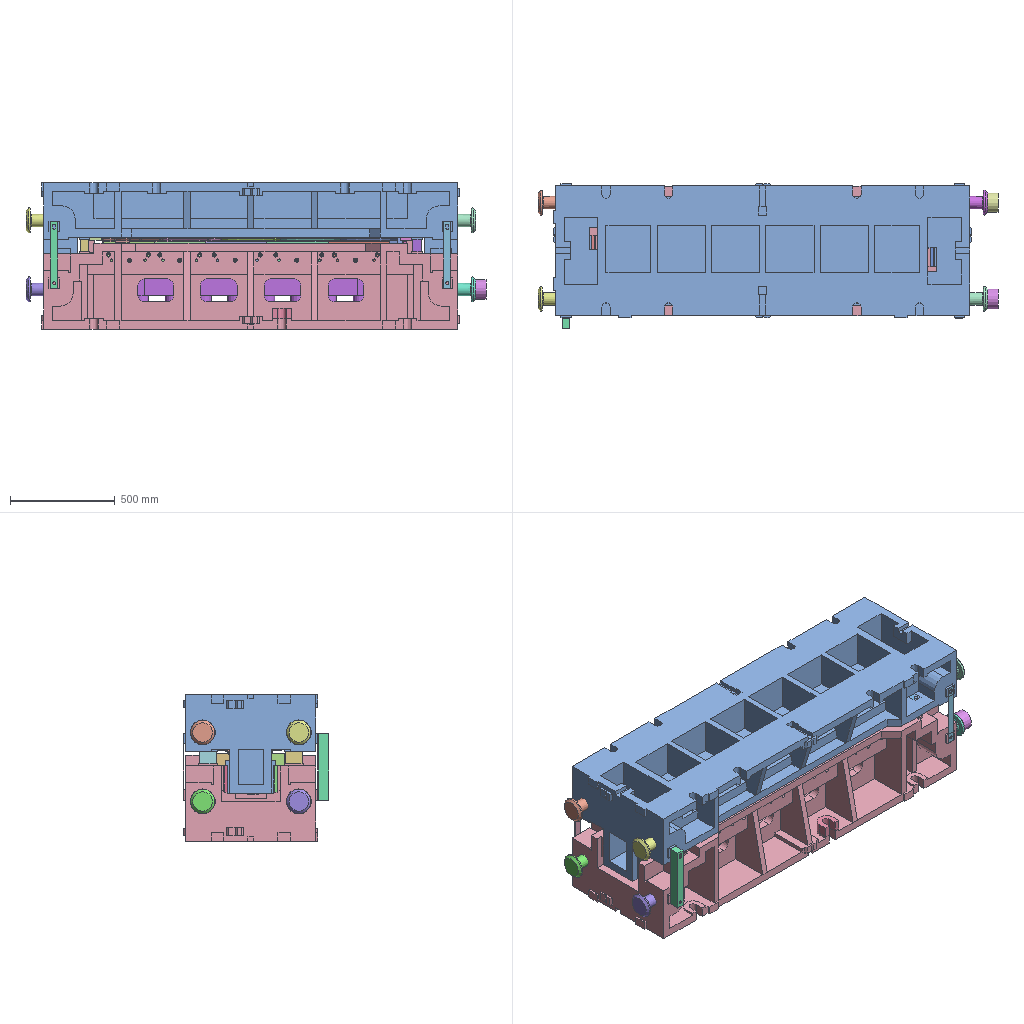Assembly | NX | 102 different items | 102 placed | box 2200 x 696 x 700 mm
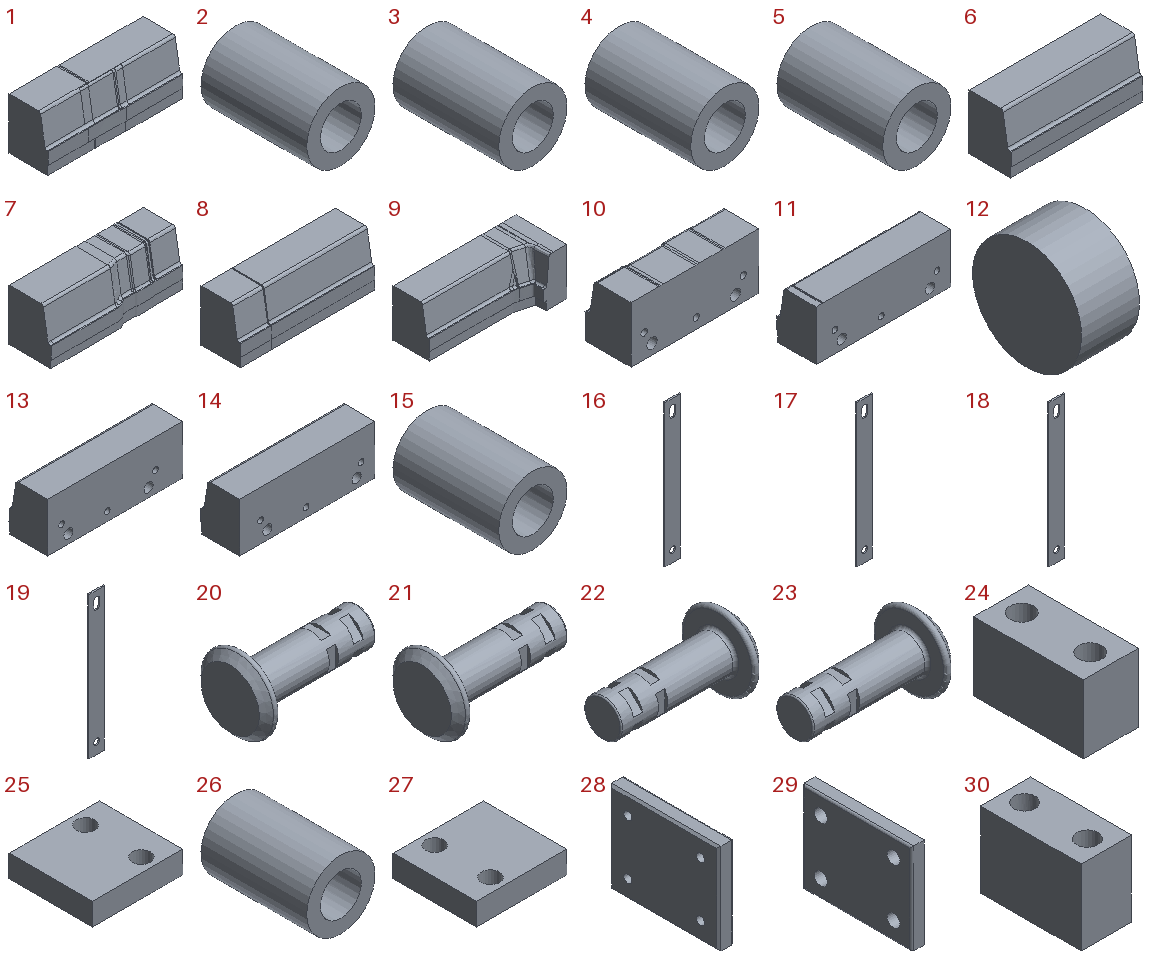Parts list (item | quantity | size | volume | features):
1 | x1 | 280 x 83.171 x 107.133 mm | 2238545 mm3 | features solid 2
2 | x1 | 20 x 31 x 20 mm | 6233 mm3 | features solid 2
3 | x1 | 20 x 31 x 20 mm | 6233 mm3 | features solid 2
4 | x1 | 20 x 31 x 20 mm | 6233 mm3 | features solid 2
5 | x1 | 20 x 31 x 20 mm | 6233 mm3 | features solid 2
6 | x1 | 255 x 82.128 x 107.133 mm | 2023073 mm3 | features solid 2
7 | x1 | 280 x 88.161 x 107.138 mm | 2308062 mm3 | features solid 2
8 | x1 | 280 x 82.346 x 107.138 mm | 2225782 mm3 | features solid 2
9 | x1 | 280 x 116 x 107.135 mm | 2471455 mm3 | features solid 2
10 | x1 | 245 x 88.207 x 107.259 mm | 2041694 mm3 | features solid 2
11 | x1 | 290 x 84.721 x 107.133 mm | 2405435 mm3 | features solid 2
12 | x1 | 50 x 94.142 x 94.142 mm | 348039 mm3 | features solid 2
13 | x1 | 295 x 84.705 x 107.133 mm | 2449051 mm3 | features solid 2
14 | x1 | 295 x 84.706 x 107.133 mm | 2449050 mm3 | features solid 2
15 | x1 | 20 x 31 x 20 mm | 6233 mm3 | features solid 2
16 | x1 | 35 x 3 x 320 mm | 32235 mm3 | features solid 2
17 | x1 | 35 x 3 x 320 mm | 32235 mm3 | features solid 2
18 | x1 | 35 x 3 x 320 mm | 32235 mm3 | features solid 2
19 | x1 | 35 x 3 x 320 mm | 32235 mm3 | features solid 2
20 | x1 | 205 x 120 x 120 mm | 705223 mm3 | features solid 2
21 | x1 | 205 x 120 x 120 mm | 705223 mm3 | features solid 2
22 | x1 | 205 x 120 x 120 mm | 705223 mm3 | features solid 2
23 | x1 | 205 x 120 x 120 mm | 705223 mm3 | features solid 2
24 | x1 | 40 x 80 x 50 mm | 137302 mm3 | features solid 2
25 | x1 | 65 x 60 x 16 mm | 58153 mm3 | features solid 2
26 | x1 | 20 x 31 x 20 mm | 6233 mm3 | features solid 2
27 | x1 | 65 x 60 x 16 mm | 58153 mm3 | features solid 2
28 | x1 | 20 x 150 x 125 mm | 356923 mm3 | features solid 2
29 | x1 | 20 x 150 x 125 mm | 356923 mm3 | features solid 2
30 | x1 | 40 x 80 x 60 mm | 176638 mm3 | features solid 2
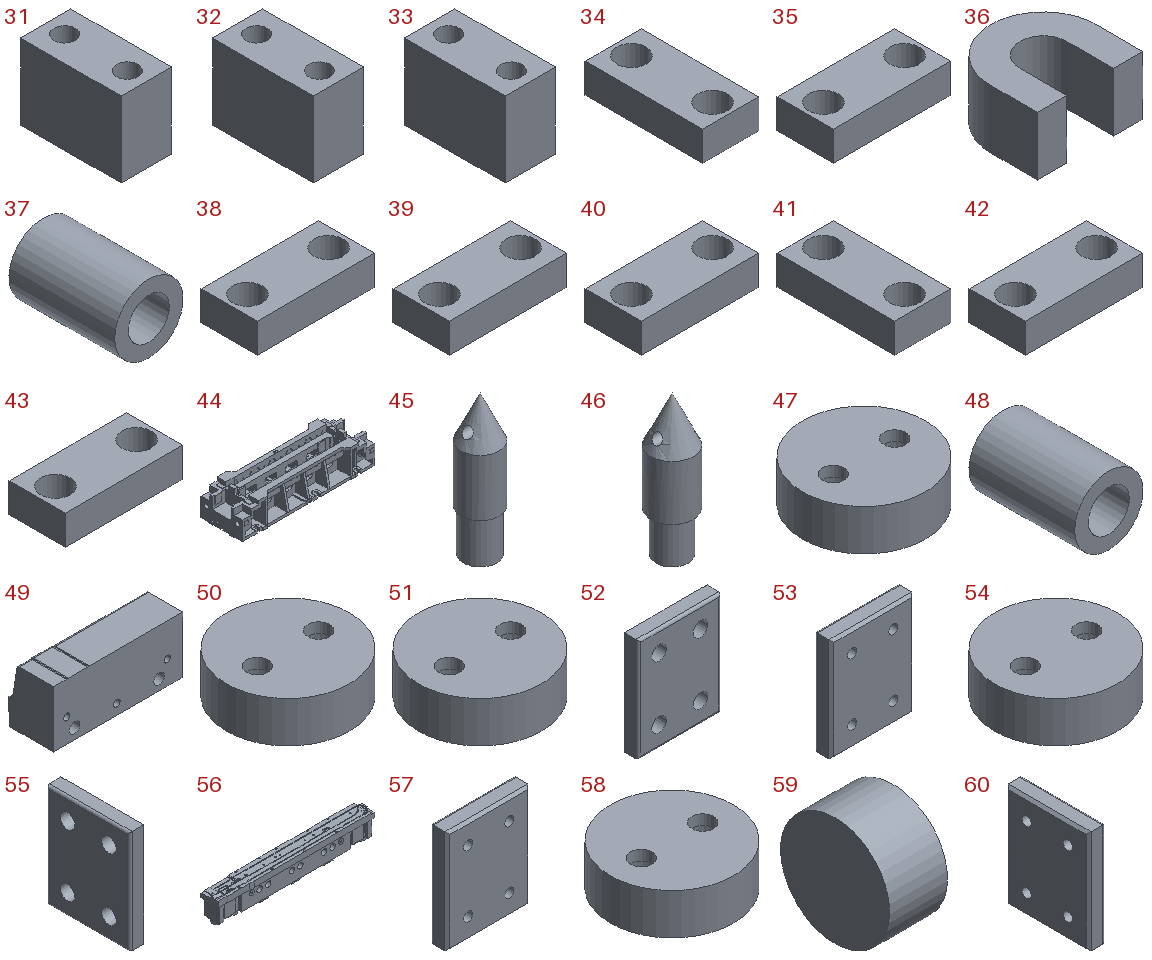31 | x1 | 40 x 80 x 60 mm | 176638 mm3 | features solid 2
32 | x1 | 40 x 80 x 60 mm | 176638 mm3 | features solid 2
33 | x1 | 40 x 80 x 60 mm | 176638 mm3 | features solid 2
34 | x1 | 38 x 80 x 20 mm | 50411 mm3 | features solid 2
35 | x1 | 80 x 38 x 20 mm | 50411 mm3 | features solid 2
36 | x1 | 90 x 85 x 50 mm | 227627 mm3 | features solid 2
37 | x1 | 20 x 31 x 20 mm | 6233 mm3 | features solid 2
38 | x1 | 80 x 38 x 20 mm | 50411 mm3 | features solid 2
39 | x1 | 80 x 38 x 20 mm | 50411 mm3 | features solid 2
40 | x1 | 80 x 38 x 20 mm | 50411 mm3 | features solid 2
41 | x1 | 38 x 80 x 20 mm | 50411 mm3 | features solid 2
42 | x1 | 80 x 38 x 20 mm | 50411 mm3 | features solid 2
43 | x1 | 80 x 38 x 20 mm | 50411 mm3 | features solid 2
44 | x1 | 2000 x 640 x 425 mm | 163390504 mm3 | features solid 2
45 | x1 | 13.7 x 13.7 x 50 mm | 5325 mm3 | features solid 2
46 | x1 | 15.7 x 15.7 x 52 mm | 6599 mm3 | features solid 2
47 | x1 | 60 x 60 x 20 mm | 48467 mm3 | features solid 2
48 | x1 | 20 x 31 x 20 mm | 6233 mm3 | features solid 2
49 | x1 | 245 x 84.473 x 107.229 mm | 2020189 mm3 | features solid 2
50 | x1 | 60 x 60 x 20 mm | 48467 mm3 | features solid 2
51 | x1 | 60 x 60 x 20 mm | 48467 mm3 | features solid 2
52 | x1 | 100 x 20 x 125 mm | 232566 mm3 | features solid 2
53 | x1 | 100 x 20 x 125 mm | 232566 mm3 | features solid 2
54 | x1 | 60 x 60 x 20 mm | 48467 mm3 | features solid 2
55 | x1 | 20 x 100 x 125 mm | 232566 mm3 | features solid 2
56 | x1 | 1460 x 169.867 x 235.617 mm | 41741038 mm3 | features solid 2
57 | x1 | 100 x 20 x 125 mm | 232566 mm3 | features solid 2
58 | x1 | 60 x 60 x 20 mm | 48467 mm3 | features solid 2
59 | x1 | 50 x 94.142 x 94.142 mm | 348039 mm3 | features solid 2
60 | x1 | 20 x 100 x 125 mm | 232566 mm3 | features solid 2
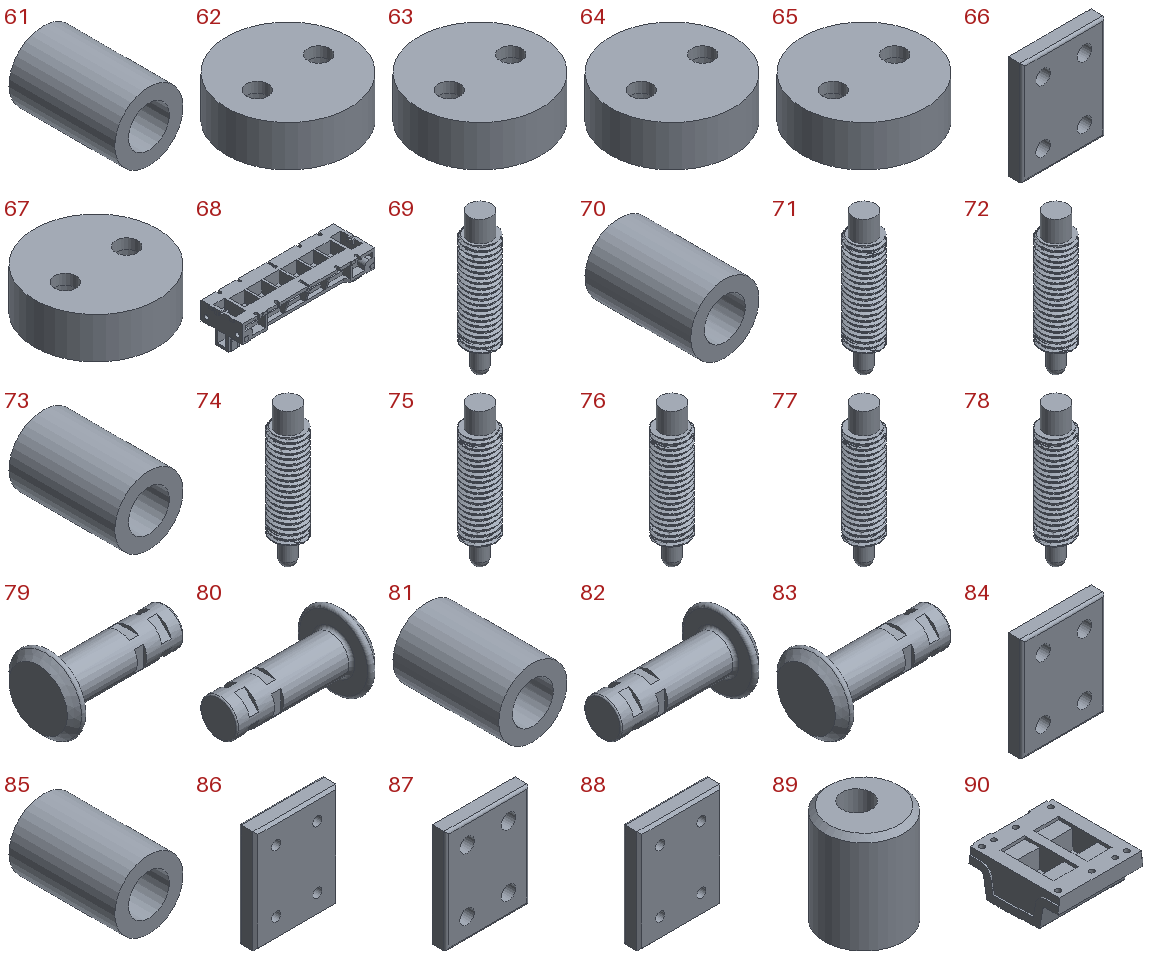61 | x1 | 20 x 31 x 20 mm | 6233 mm3 | features solid 2
62 | x1 | 60 x 60 x 20 mm | 48467 mm3 | features solid 2
63 | x1 | 60 x 60 x 20 mm | 48467 mm3 | features solid 2
64 | x1 | 60 x 60 x 20 mm | 48467 mm3 | features solid 2
65 | x1 | 60 x 60 x 20 mm | 48467 mm3 | features solid 2
66 | x1 | 100 x 20 x 125 mm | 232566 mm3 | features solid 2
67 | x1 | 60 x 60 x 20 mm | 48467 mm3 | features solid 2
68 | x1 | 2000 x 640 x 475 mm | 146467854 mm3 | features solid 2
69 | x1 | 11.998 x 11.997 x 53 mm | 4026 mm3 | features solid 2
70 | x1 | 20 x 31 x 20 mm | 6233 mm3 | features solid 2
71 | x1 | 11.998 x 11.997 x 53 mm | 4026 mm3 | features solid 2
72 | x1 | 11.998 x 11.997 x 53 mm | 4026 mm3 | features solid 2
73 | x1 | 20 x 31 x 20 mm | 6233 mm3 | features solid 2
74 | x1 | 11.998 x 11.997 x 53 mm | 4026 mm3 | features solid 2
75 | x1 | 11.998 x 11.997 x 53 mm | 4026 mm3 | features solid 2
76 | x1 | 11.998 x 11.997 x 53 mm | 4026 mm3 | features solid 2
77 | x1 | 11.998 x 11.997 x 53 mm | 4026 mm3 | features solid 2
78 | x1 | 11.998 x 11.997 x 53 mm | 4026 mm3 | features solid 2
79 | x1 | 205 x 120 x 120 mm | 705223 mm3 | features solid 2
80 | x1 | 205 x 120 x 120 mm | 705223 mm3 | features solid 2
81 | x1 | 20 x 31 x 20 mm | 6233 mm3 | features solid 2
82 | x1 | 205 x 120 x 120 mm | 705223 mm3 | features solid 2
83 | x1 | 205 x 120 x 120 mm | 705223 mm3 | features solid 2
84 | x1 | 100 x 20 x 125 mm | 232566 mm3 | features solid 2
85 | x1 | 20 x 31 x 20 mm | 6233 mm3 | features solid 2
86 | x1 | 100 x 20 x 125 mm | 232566 mm3 | features solid 2
87 | x1 | 100 x 20 x 125 mm | 232566 mm3 | features solid 2
88 | x1 | 100 x 20 x 125 mm | 232566 mm3 | features solid 2
89 | x1 | 16 x 16 x 20.5 mm | 3091 mm3 | features solid 2
90 | x1 | 290 x 310 x 126.004 mm | 6972719 mm3 | features solid 2
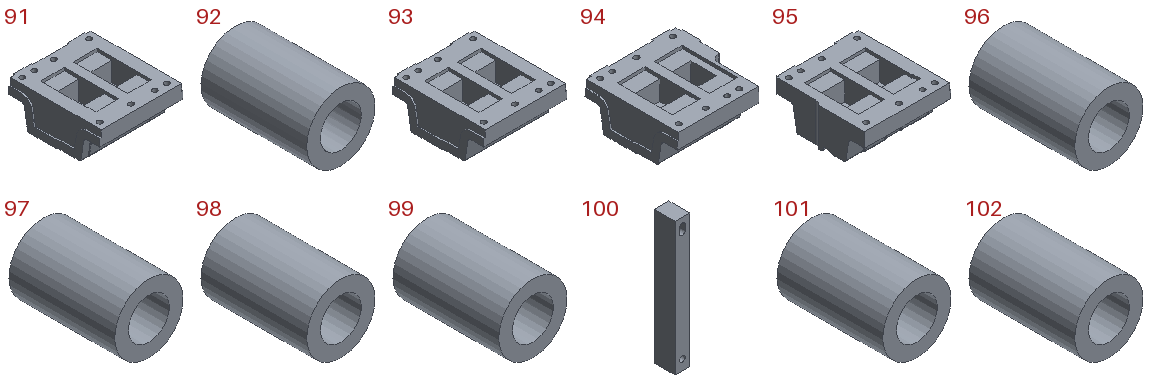91 | x1 | 280 x 310 x 126.004 mm | 6755474 mm3 | features solid 2
92 | x1 | 20 x 31 x 20 mm | 6233 mm3 | features solid 2
93 | x1 | 280.327 x 310 x 126.004 mm | 6770468 mm3 | features solid 2
94 | x1 | 305 x 310 x 125.996 mm | 6792553 mm3 | features solid 2
95 | x1 | 290 x 310 x 129.453 mm | 6859880 mm3 | features solid 2
96 | x1 | 20 x 31 x 20 mm | 6233 mm3 | features solid 2
97 | x1 | 20 x 31 x 20 mm | 6233 mm3 | features solid 2
98 | x1 | 20 x 31 x 20 mm | 6233 mm3 | features solid 2
99 | x1 | 20 x 31 x 20 mm | 6233 mm3 | features solid 2
100 | x1 | 35 x 50 x 320 mm | 537249 mm3 | features solid 2
101 | x1 | 20 x 31 x 20 mm | 6233 mm3 | features solid 2
102 | x1 | 20 x 31 x 20 mm | 6233 mm3 | features solid 2